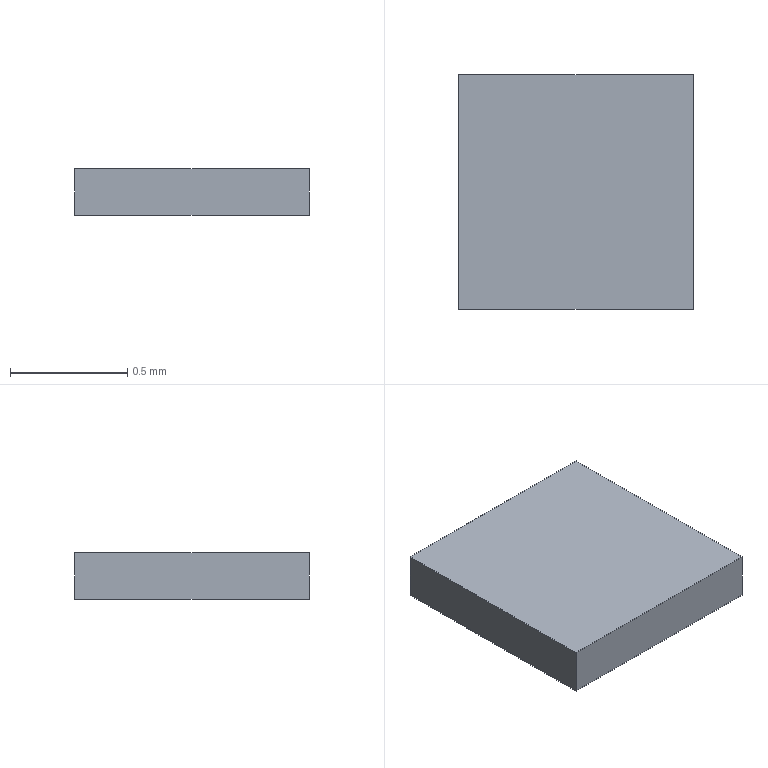Part | Creo | 1 solid | 6 faces | box 1 x 1 x 0.2 mm | volume 0.2 mm3 | plane 6
STEP:
#1=CARTESIAN_POINT('',(0.,0.,0.));
#2=DIRECTION('',(0.,0.,1.));
#3=DIRECTION('',(1.,0.,0.));
#4=AXIS2_PLACEMENT_3D('',#1,#2,#3);
#5=CARTESIAN_POINT('',(-0.5,-0.5,0.));
#6=VERTEX_POINT('',#5);
#7=CARTESIAN_POINT('',(0.5,-0.5,0.));
#8=VERTEX_POINT('',#7);
#9=CARTESIAN_POINT('',(-0.5,-0.5,0.));
#10=DIRECTION('',(1.,0.,0.));
#11=VECTOR('',#10,1.);
#12=LINE('',#9,#11);
#13=EDGE_CURVE('',#6,#8,#12,.T.);
#14=ORIENTED_EDGE('',*,*,#13,.T.);
#15=CARTESIAN_POINT('',(0.5,0.5,0.));
#16=VERTEX_POINT('',#15);
#17=CARTESIAN_POINT('',(0.5,-0.5,0.));
#18=DIRECTION('',(0.,1.,0.));
#19=VECTOR('',#18,1.);
#20=LINE('',#17,#19);
#21=EDGE_CURVE('',#8,#16,#20,.T.);
#22=ORIENTED_EDGE('',*,*,#21,.T.);
#23=CARTESIAN_POINT('',(-0.5,0.5,0.));
#24=VERTEX_POINT('',#23);
#25=CARTESIAN_POINT('',(0.5,0.5,0.));
#26=DIRECTION('',(-1.,0.,0.));
#27=VECTOR('',#26,1.);
#28=LINE('',#25,#27);
#29=EDGE_CURVE('',#16,#24,#28,.T.);
#30=ORIENTED_EDGE('',*,*,#29,.T.);
#31=CARTESIAN_POINT('',(-0.5,0.5,0.));
#32=DIRECTION('',(0.,-1.,0.));
#33=VECTOR('',#32,1.);
#34=LINE('',#31,#33);
#35=EDGE_CURVE('',#24,#6,#34,.T.);
#36=ORIENTED_EDGE('',*,*,#35,.T.);
#37=EDGE_LOOP('',(#14,#22,#30,#36));
#38=FACE_OUTER_BOUND('',#37,.F.);
#39=CARTESIAN_POINT('',(0.,0.,0.));
#40=DIRECTION('',(0.,0.,1.));
#41=DIRECTION('',(1.,0.,0.));
#42=AXIS2_PLACEMENT_3D('',#39,#40,#41);
#43=PLANE('',#42);
#44=ADVANCED_FACE('',(#38),#43,.F.);
#45=ORIENTED_EDGE('',*,*,#13,.F.);
#46=CARTESIAN_POINT('',(-0.5,-0.5,0.2));
#47=VERTEX_POINT('',#46);
#48=CARTESIAN_POINT('',(-0.5,-0.5,0.));
#49=DIRECTION('',(0.,0.,1.));
#50=VECTOR('',#49,0.2);
#51=LINE('',#48,#50);
#52=EDGE_CURVE('',#6,#47,#51,.T.);
#53=ORIENTED_EDGE('',*,*,#52,.T.);
#54=CARTESIAN_POINT('',(0.5,-0.5,0.2));
#55=VERTEX_POINT('',#54);
#56=CARTESIAN_POINT('',(-0.5,-0.5,0.2));
#57=DIRECTION('',(1.,0.,0.));
#58=VECTOR('',#57,1.);
#59=LINE('',#56,#58);
#60=EDGE_CURVE('',#47,#55,#59,.T.);
#61=ORIENTED_EDGE('',*,*,#60,.T.);
#62=CARTESIAN_POINT('',(0.5,-0.5,0.));
#63=DIRECTION('',(0.,0.,1.));
#64=VECTOR('',#63,0.2);
#65=LINE('',#62,#64);
#66=EDGE_CURVE('',#8,#55,#65,.T.);
#67=ORIENTED_EDGE('',*,*,#66,.F.);
#68=EDGE_LOOP('',(#45,#53,#61,#67));
#69=FACE_OUTER_BOUND('',#68,.F.);
#70=CARTESIAN_POINT('',(-0.5,-0.5,0.));
#71=DIRECTION('',(0.,-1.,0.));
#72=DIRECTION('',(1.,0.,0.));
#73=AXIS2_PLACEMENT_3D('',#70,#71,#72);
#74=PLANE('',#73);
#75=ADVANCED_FACE('',(#69),#74,.T.);
#76=ORIENTED_EDGE('',*,*,#35,.F.);
#77=CARTESIAN_POINT('',(-0.5,0.5,0.2));
#78=VERTEX_POINT('',#77);
#79=CARTESIAN_POINT('',(-0.5,0.5,0.));
#80=DIRECTION('',(0.,0.,1.));
#81=VECTOR('',#80,0.2);
#82=LINE('',#79,#81);
#83=EDGE_CURVE('',#24,#78,#82,.T.);
#84=ORIENTED_EDGE('',*,*,#83,.T.);
#85=CARTESIAN_POINT('',(-0.5,0.5,0.2));
#86=DIRECTION('',(0.,-1.,0.));
#87=VECTOR('',#86,1.);
#88=LINE('',#85,#87);
#89=EDGE_CURVE('',#78,#47,#88,.T.);
#90=ORIENTED_EDGE('',*,*,#89,.T.);
#91=ORIENTED_EDGE('',*,*,#52,.F.);
#92=EDGE_LOOP('',(#76,#84,#90,#91));
#93=FACE_OUTER_BOUND('',#92,.F.);
#94=CARTESIAN_POINT('',(-0.5,0.5,0.));
#95=DIRECTION('',(-1.,0.,0.));
#96=DIRECTION('',(0.,-1.,0.));
#97=AXIS2_PLACEMENT_3D('',#94,#95,#96);
#98=PLANE('',#97);
#99=ADVANCED_FACE('',(#93),#98,.T.);
#100=ORIENTED_EDGE('',*,*,#29,.F.);
#101=CARTESIAN_POINT('',(0.5,0.5,0.2));
#102=VERTEX_POINT('',#101);
#103=CARTESIAN_POINT('',(0.5,0.5,0.));
#104=DIRECTION('',(0.,0.,1.));
#105=VECTOR('',#104,0.2);
#106=LINE('',#103,#105);
#107=EDGE_CURVE('',#16,#102,#106,.T.);
#108=ORIENTED_EDGE('',*,*,#107,.T.);
#109=CARTESIAN_POINT('',(0.5,0.5,0.2));
#110=DIRECTION('',(-1.,0.,0.));
#111=VECTOR('',#110,1.);
#112=LINE('',#109,#111);
#113=EDGE_CURVE('',#102,#78,#112,.T.);
#114=ORIENTED_EDGE('',*,*,#113,.T.);
#115=ORIENTED_EDGE('',*,*,#83,.F.);
#116=EDGE_LOOP('',(#100,#108,#114,#115));
#117=FACE_OUTER_BOUND('',#116,.F.);
#118=CARTESIAN_POINT('',(0.5,0.5,0.));
#119=DIRECTION('',(0.,1.,0.));
#120=DIRECTION('',(-1.,0.,0.));
#121=AXIS2_PLACEMENT_3D('',#118,#119,#120);
#122=PLANE('',#121);
#123=ADVANCED_FACE('',(#117),#122,.T.);
#124=ORIENTED_EDGE('',*,*,#21,.F.);
#125=ORIENTED_EDGE('',*,*,#66,.T.);
#126=CARTESIAN_POINT('',(0.5,-0.5,0.2));
#127=DIRECTION('',(0.,1.,0.));
#128=VECTOR('',#127,1.);
#129=LINE('',#126,#128);
#130=EDGE_CURVE('',#55,#102,#129,.T.);
#131=ORIENTED_EDGE('',*,*,#130,.T.);
#132=ORIENTED_EDGE('',*,*,#107,.F.);
#133=EDGE_LOOP('',(#124,#125,#131,#132));
#134=FACE_OUTER_BOUND('',#133,.F.);
#135=CARTESIAN_POINT('',(0.5,-0.5,0.));
#136=DIRECTION('',(1.,0.,0.));
#137=DIRECTION('',(0.,1.,0.));
#138=AXIS2_PLACEMENT_3D('',#135,#136,#137);
#139=PLANE('',#138);
#140=ADVANCED_FACE('',(#134),#139,.T.);
#141=ORIENTED_EDGE('',*,*,#60,.F.);
#142=ORIENTED_EDGE('',*,*,#89,.F.);
#143=ORIENTED_EDGE('',*,*,#113,.F.);
#144=ORIENTED_EDGE('',*,*,#130,.F.);
#145=EDGE_LOOP('',(#141,#142,#143,#144));
#146=FACE_OUTER_BOUND('',#145,.F.);
#147=CARTESIAN_POINT('',(0.,0.,0.2));
#148=DIRECTION('',(0.,0.,1.));
#149=DIRECTION('',(1.,0.,0.));
#150=AXIS2_PLACEMENT_3D('',#147,#148,#149);
#151=PLANE('',#150);
#152=ADVANCED_FACE('',(#146),#151,.T.);
#153=CLOSED_SHELL('',(#44,#75,#99,#123,#140,#152));
#154=MANIFOLD_SOLID_BREP('',#153);
#155=(LENGTH_UNIT()NAMED_UNIT(*)SI_UNIT(.MILLI.,.METRE.));
#156=UNCERTAINTY_MEASURE_WITH_UNIT(LENGTH_MEASURE(0.0001428),#155,'','');
#157=(NAMED_UNIT(*)PLANE_ANGLE_UNIT()SI_UNIT($,.RADIAN.));
#158=PLANE_ANGLE_MEASURE_WITH_UNIT(PLANE_ANGLE_MEASURE(0.01745),#157);
#159=(CONVERSION_BASED_UNIT('DEGREE',#158)NAMED_UNIT(*)PLANE_ANGLE_UNIT());
#160=(NAMED_UNIT(*)SI_UNIT($,.STERADIAN.)SOLID_ANGLE_UNIT());
#161=(GEOMETRIC_REPRESENTATION_CONTEXT(3)GLOBAL_UNCERTAINTY_ASSIGNED_CONTEXT((#156))GLOBAL_UNIT_ASSIGNED_CONTEXT((#155,#159,#160))REPRESENTATION_CONTEXT('',''));
#162=ADVANCED_BREP_SHAPE_REPRESENTATION('',(#4,#154),#161);